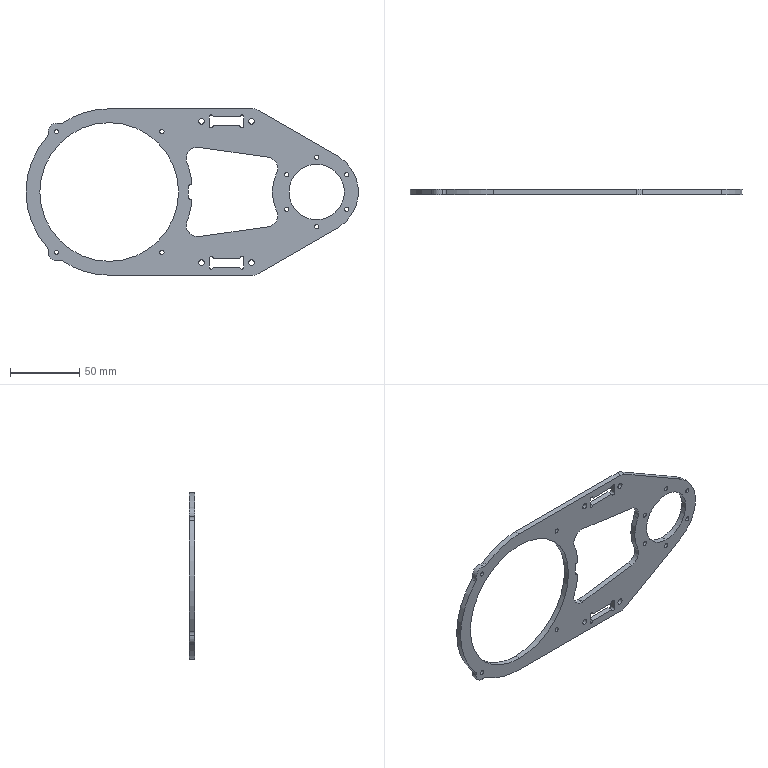Part | SolidWorks | features Fillet 3, Extrusion 1 | 1 solid | 89 faces | box 239.599 x 4 x 120 mm | volume 43541 mm3 | cylinder 71 | plane 18 | commonest cylinder face diameters 3.2 x20 3 x12 4.2 x8 16 x7 6 x5 120 x5